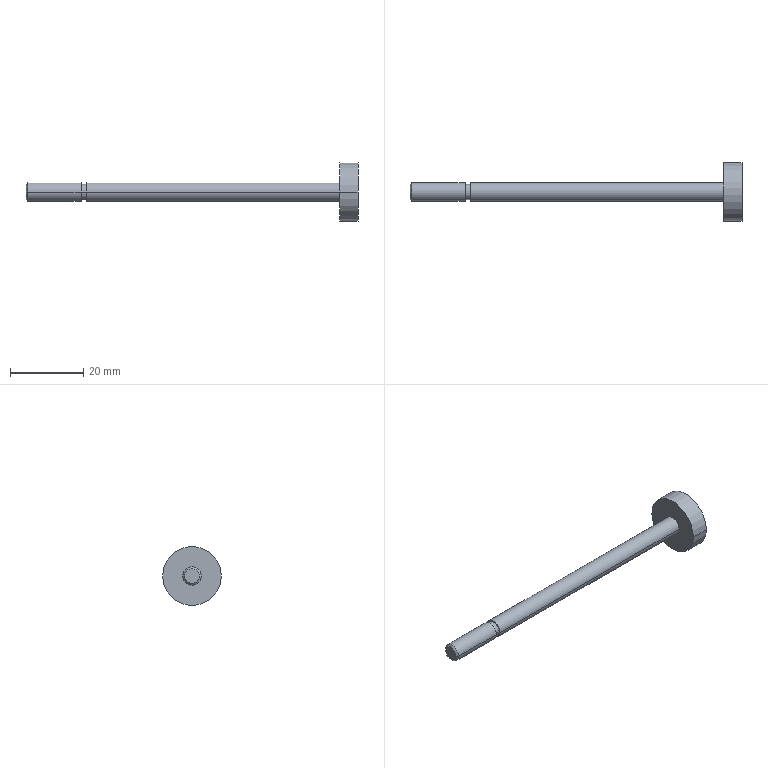Part | SolidWorks | features RefAxis 12, 3DProfileFeature 4, Revolution 1 | 1 solid | 15 faces | box 90.5 x 16 x 16 mm | volume 2673 mm3 | cylinder 8 | plane 5 | cone 2 | commonest cylinder face diameters 5 x4 4.13 x2 16 x2
STEP:
#1=CARTESIAN_POINT('',(90.5,-8.,0.));
#2=VERTEX_POINT('',#1);
#3=CARTESIAN_POINT('',(90.5,8.,0.));
#4=VERTEX_POINT('',#3);
#5=CARTESIAN_POINT('',(90.5,0.,0.));
#6=DIRECTION('',(-1.,0.,0.));
#7=DIRECTION('',(0.,-1.,0.));
#8=AXIS2_PLACEMENT_3D('',#5,#6,#7);
#9=CIRCLE('',#8,8.);
#10=EDGE_CURVE('',#2,#4,#9,.T.);
#11=ORIENTED_EDGE('',*,*,#10,.T.);
#12=CARTESIAN_POINT('',(85.5,8.,0.));
#13=VERTEX_POINT('',#12);
#14=CARTESIAN_POINT('',(90.5,8.,0.));
#15=DIRECTION('',(-1.,0.,0.));
#16=VECTOR('',#15,1000.);
#17=LINE('',#14,#16);
#18=EDGE_CURVE('',#4,#13,#17,.T.);
#19=ORIENTED_EDGE('',*,*,#18,.T.);
#20=CARTESIAN_POINT('',(85.5,-8.,0.));
#21=VERTEX_POINT('',#20);
#22=CARTESIAN_POINT('',(85.5,0.,0.));
#23=DIRECTION('',(-1.,0.,0.));
#24=DIRECTION('',(0.,-1.,0.));
#25=AXIS2_PLACEMENT_3D('',#22,#23,#24);
#26=CIRCLE('',#25,8.);
#27=EDGE_CURVE('',#21,#13,#26,.T.);
#28=ORIENTED_EDGE('',*,*,#27,.F.);
#29=CARTESIAN_POINT('',(90.5,-8.,0.));
#30=DIRECTION('',(-1.,0.,0.));
#31=VECTOR('',#30,1000.);
#32=LINE('',#29,#31);
#33=EDGE_CURVE('',#2,#21,#32,.T.);
#34=ORIENTED_EDGE('',*,*,#33,.F.);
#35=EDGE_LOOP('',(#11,#19,#28,#34));
#36=FACE_OUTER_BOUND('',#35,.T.);
#37=CARTESIAN_POINT('',(90.5,0.,0.));
#38=DIRECTION('',(-1.,0.,0.));
#39=DIRECTION('',(0.,-1.,0.));
#40=AXIS2_PLACEMENT_3D('',#37,#38,#39);
#41=CYLINDRICAL_SURFACE('',#40,8.);
#42=ADVANCED_FACE('',(#36),#41,.T.);
#43=CARTESIAN_POINT('',(85.5,-2.5,0.));
#44=VERTEX_POINT('',#43);
#45=CARTESIAN_POINT('',(85.5,2.5,0.));
#46=VERTEX_POINT('',#45);
#47=CARTESIAN_POINT('',(85.5,0.,0.));
#48=DIRECTION('',(-1.,0.,0.));
#49=DIRECTION('',(0.,-1.,0.));
#50=AXIS2_PLACEMENT_3D('',#47,#48,#49);
#51=CIRCLE('',#50,2.5);
#52=EDGE_CURVE('',#44,#46,#51,.T.);
#53=ORIENTED_EDGE('',*,*,#52,.T.);
#54=CARTESIAN_POINT('',(16.5,2.5,0.));
#55=VERTEX_POINT('',#54);
#56=CARTESIAN_POINT('',(90.5,2.5,0.));
#57=DIRECTION('',(-1.,0.,0.));
#58=VECTOR('',#57,1000.);
#59=LINE('',#56,#58);
#60=EDGE_CURVE('',#46,#55,#59,.T.);
#61=ORIENTED_EDGE('',*,*,#60,.T.);
#62=CARTESIAN_POINT('',(16.5,-2.5,0.));
#63=VERTEX_POINT('',#62);
#64=CARTESIAN_POINT('',(16.5,0.,0.));
#65=DIRECTION('',(-1.,0.,0.));
#66=DIRECTION('',(0.,-1.,0.));
#67=AXIS2_PLACEMENT_3D('',#64,#65,#66);
#68=CIRCLE('',#67,2.5);
#69=EDGE_CURVE('',#63,#55,#68,.T.);
#70=ORIENTED_EDGE('',*,*,#69,.F.);
#71=CARTESIAN_POINT('',(90.5,-2.5,0.));
#72=DIRECTION('',(-1.,0.,0.));
#73=VECTOR('',#72,1000.);
#74=LINE('',#71,#73);
#75=EDGE_CURVE('',#44,#63,#74,.T.);
#76=ORIENTED_EDGE('',*,*,#75,.F.);
#77=EDGE_LOOP('',(#53,#61,#70,#76));
#78=FACE_OUTER_BOUND('',#77,.T.);
#79=CARTESIAN_POINT('',(90.5,0.,0.));
#80=DIRECTION('',(-1.,0.,0.));
#81=DIRECTION('',(0.,-1.,0.));
#82=AXIS2_PLACEMENT_3D('',#79,#80,#81);
#83=CYLINDRICAL_SURFACE('',#82,2.5);
#84=ADVANCED_FACE('',(#78),#83,.T.);
#85=CARTESIAN_POINT('',(16.5,-2.065,0.));
#86=VERTEX_POINT('',#85);
#87=CARTESIAN_POINT('',(16.5,2.065,0.));
#88=VERTEX_POINT('',#87);
#89=CARTESIAN_POINT('',(16.5,0.,0.));
#90=DIRECTION('',(-1.,0.,0.));
#91=DIRECTION('',(0.,-1.,0.));
#92=AXIS2_PLACEMENT_3D('',#89,#90,#91);
#93=CIRCLE('',#92,2.065);
#94=EDGE_CURVE('',#86,#88,#93,.T.);
#95=ORIENTED_EDGE('',*,*,#94,.T.);
#96=CARTESIAN_POINT('',(15.,2.065,0.));
#97=VERTEX_POINT('',#96);
#98=CARTESIAN_POINT('',(90.5,2.065,0.));
#99=DIRECTION('',(-1.,0.,0.));
#100=VECTOR('',#99,1000.);
#101=LINE('',#98,#100);
#102=EDGE_CURVE('',#88,#97,#101,.T.);
#103=ORIENTED_EDGE('',*,*,#102,.T.);
#104=CARTESIAN_POINT('',(15.,-2.065,0.));
#105=VERTEX_POINT('',#104);
#106=CARTESIAN_POINT('',(15.,0.,0.));
#107=DIRECTION('',(-1.,0.,0.));
#108=DIRECTION('',(0.,-1.,0.));
#109=AXIS2_PLACEMENT_3D('',#106,#107,#108);
#110=CIRCLE('',#109,2.065);
#111=EDGE_CURVE('',#105,#97,#110,.T.);
#112=ORIENTED_EDGE('',*,*,#111,.F.);
#113=CARTESIAN_POINT('',(90.5,-2.065,0.));
#114=DIRECTION('',(-1.,0.,0.));
#115=VECTOR('',#114,1000.);
#116=LINE('',#113,#115);
#117=EDGE_CURVE('',#86,#105,#116,.T.);
#118=ORIENTED_EDGE('',*,*,#117,.F.);
#119=EDGE_LOOP('',(#95,#103,#112,#118));
#120=FACE_OUTER_BOUND('',#119,.T.);
#121=CARTESIAN_POINT('',(90.5,0.,0.));
#122=DIRECTION('',(-1.,0.,0.));
#123=DIRECTION('',(0.,-1.,0.));
#124=AXIS2_PLACEMENT_3D('',#121,#122,#123);
#125=CYLINDRICAL_SURFACE('',#124,2.065);
#126=ADVANCED_FACE('',(#120),#125,.T.);
#127=CARTESIAN_POINT('',(15.,-2.5,0.));
#128=VERTEX_POINT('',#127);
#129=CARTESIAN_POINT('',(15.,2.5,0.));
#130=VERTEX_POINT('',#129);
#131=CARTESIAN_POINT('',(15.,0.,0.));
#132=DIRECTION('',(-1.,0.,0.));
#133=DIRECTION('',(0.,-1.,0.));
#134=AXIS2_PLACEMENT_3D('',#131,#132,#133);
#135=CIRCLE('',#134,2.5);
#136=EDGE_CURVE('',#128,#130,#135,.T.);
#137=ORIENTED_EDGE('',*,*,#136,.T.);
#138=CARTESIAN_POINT('',(0.4905,2.5,0.));
#139=VERTEX_POINT('',#138);
#140=CARTESIAN_POINT('',(90.5,2.5,0.));
#141=DIRECTION('',(-1.,0.,0.));
#142=VECTOR('',#141,1000.);
#143=LINE('',#140,#142);
#144=EDGE_CURVE('',#130,#139,#143,.T.);
#145=ORIENTED_EDGE('',*,*,#144,.T.);
#146=CARTESIAN_POINT('',(0.4905,-2.5,0.));
#147=VERTEX_POINT('',#146);
#148=CARTESIAN_POINT('',(0.4905,0.,0.));
#149=DIRECTION('',(-1.,0.,0.));
#150=DIRECTION('',(0.,-1.,0.));
#151=AXIS2_PLACEMENT_3D('',#148,#149,#150);
#152=CIRCLE('',#151,2.5);
#153=EDGE_CURVE('',#147,#139,#152,.T.);
#154=ORIENTED_EDGE('',*,*,#153,.F.);
#155=CARTESIAN_POINT('',(90.5,-2.5,0.));
#156=DIRECTION('',(-1.,0.,0.));
#157=VECTOR('',#156,1000.);
#158=LINE('',#155,#157);
#159=EDGE_CURVE('',#128,#147,#158,.T.);
#160=ORIENTED_EDGE('',*,*,#159,.F.);
#161=EDGE_LOOP('',(#137,#145,#154,#160));
#162=FACE_OUTER_BOUND('',#161,.T.);
#163=CARTESIAN_POINT('',(90.5,0.,0.));
#164=DIRECTION('',(-1.,0.,0.));
#165=DIRECTION('',(0.,-1.,0.));
#166=AXIS2_PLACEMENT_3D('',#163,#164,#165);
#167=CYLINDRICAL_SURFACE('',#166,2.5);
#168=ADVANCED_FACE('',(#162),#167,.T.);
#169=CARTESIAN_POINT('',(0.,-2.01,0.));
#170=VERTEX_POINT('',#169);
#171=CARTESIAN_POINT('',(0.,2.01,0.));
#172=VERTEX_POINT('',#171);
#173=CARTESIAN_POINT('',(0.,0.,0.));
#174=DIRECTION('',(-1.,0.,0.));
#175=DIRECTION('',(0.,-1.,0.));
#176=AXIS2_PLACEMENT_3D('',#173,#174,#175);
#177=CIRCLE('',#176,2.01);
#178=EDGE_CURVE('',#170,#172,#177,.T.);
#179=ORIENTED_EDGE('',*,*,#178,.F.);
#180=CARTESIAN_POINT('',(0.4905,-2.5,0.));
#181=DIRECTION('',(0.7071,-0.7071,0.));
#182=VECTOR('',#181,1000.);
#183=LINE('',#180,#182);
#184=EDGE_CURVE('',#170,#147,#183,.T.);
#185=ORIENTED_EDGE('',*,*,#184,.T.);
#186=ORIENTED_EDGE('',*,*,#153,.T.);
#187=CARTESIAN_POINT('',(0.4905,2.5,0.));
#188=DIRECTION('',(0.7071,0.7071,0.));
#189=VECTOR('',#188,1000.);
#190=LINE('',#187,#189);
#191=EDGE_CURVE('',#172,#139,#190,.T.);
#192=ORIENTED_EDGE('',*,*,#191,.F.);
#193=EDGE_LOOP('',(#179,#185,#186,#192));
#194=FACE_OUTER_BOUND('',#193,.T.);
#195=CARTESIAN_POINT('',(0.4905,0.,0.));
#196=DIRECTION('',(1.,0.,0.));
#197=DIRECTION('',(0.,1.,0.));
#198=AXIS2_PLACEMENT_3D('',#195,#196,#197);
#199=CONICAL_SURFACE('',#198,2.5,0.7854);
#200=ADVANCED_FACE('',(#194),#199,.T.);
#201=CARTESIAN_POINT('',(0.,0.,0.));
#202=DIRECTION('',(-1.,0.,0.));
#203=DIRECTION('',(0.,-1.,0.));
#204=AXIS2_PLACEMENT_3D('',#201,#202,#203);
#205=CIRCLE('',#204,2.01);
#206=EDGE_CURVE('',#172,#170,#205,.T.);
#207=ORIENTED_EDGE('',*,*,#206,.T.);
#208=ORIENTED_EDGE('',*,*,#178,.T.);
#209=EDGE_LOOP('',(#207,#208));
#210=FACE_OUTER_BOUND('',#209,.T.);
#211=CARTESIAN_POINT('',(0.,0.,0.));
#212=DIRECTION('',(1.,0.,0.));
#213=DIRECTION('',(0.,1.,0.));
#214=AXIS2_PLACEMENT_3D('',#211,#212,#213);
#215=PLANE('',#214);
#216=ADVANCED_FACE('',(#210),#215,.F.);
#217=ORIENTED_EDGE('',*,*,#184,.F.);
#218=ORIENTED_EDGE('',*,*,#206,.F.);
#219=ORIENTED_EDGE('',*,*,#191,.T.);
#220=CARTESIAN_POINT('',(0.4905,0.,0.));
#221=DIRECTION('',(-1.,0.,0.));
#222=DIRECTION('',(0.,-1.,0.));
#223=AXIS2_PLACEMENT_3D('',#220,#221,#222);
#224=CIRCLE('',#223,2.5);
#225=EDGE_CURVE('',#139,#147,#224,.T.);
#226=ORIENTED_EDGE('',*,*,#225,.T.);
#227=EDGE_LOOP('',(#217,#218,#219,#226));
#228=FACE_OUTER_BOUND('',#227,.T.);
#229=CARTESIAN_POINT('',(0.4905,0.,0.));
#230=DIRECTION('',(1.,0.,0.));
#231=DIRECTION('',(0.,1.,0.));
#232=AXIS2_PLACEMENT_3D('',#229,#230,#231);
#233=CONICAL_SURFACE('',#232,2.5,0.7854);
#234=ADVANCED_FACE('',(#228),#233,.T.);
#235=ORIENTED_EDGE('',*,*,#144,.F.);
#236=CARTESIAN_POINT('',(15.,0.,0.));
#237=DIRECTION('',(-1.,0.,0.));
#238=DIRECTION('',(0.,-1.,0.));
#239=AXIS2_PLACEMENT_3D('',#236,#237,#238);
#240=CIRCLE('',#239,2.5);
#241=EDGE_CURVE('',#130,#128,#240,.T.);
#242=ORIENTED_EDGE('',*,*,#241,.T.);
#243=ORIENTED_EDGE('',*,*,#159,.T.);
#244=ORIENTED_EDGE('',*,*,#225,.F.);
#245=EDGE_LOOP('',(#235,#242,#243,#244));
#246=FACE_OUTER_BOUND('',#245,.T.);
#247=CARTESIAN_POINT('',(90.5,0.,0.));
#248=DIRECTION('',(-1.,0.,0.));
#249=DIRECTION('',(0.,-1.,0.));
#250=AXIS2_PLACEMENT_3D('',#247,#248,#249);
#251=CYLINDRICAL_SURFACE('',#250,2.5);
#252=ADVANCED_FACE('',(#246),#251,.T.);
#253=ORIENTED_EDGE('',*,*,#136,.F.);
#254=ORIENTED_EDGE('',*,*,#241,.F.);
#255=EDGE_LOOP('',(#253,#254));
#256=FACE_OUTER_BOUND('',#255,.T.);
#257=ORIENTED_EDGE('',*,*,#111,.T.);
#258=CARTESIAN_POINT('',(15.,0.,0.));
#259=DIRECTION('',(-1.,0.,0.));
#260=DIRECTION('',(0.,-1.,0.));
#261=AXIS2_PLACEMENT_3D('',#258,#259,#260);
#262=CIRCLE('',#261,2.065);
#263=EDGE_CURVE('',#97,#105,#262,.T.);
#264=ORIENTED_EDGE('',*,*,#263,.T.);
#265=EDGE_LOOP('',(#257,#264));
#266=FACE_BOUND('',#265,.T.);
#267=CARTESIAN_POINT('',(15.,2.5,0.));
#268=DIRECTION('',(-1.,0.,0.));
#269=DIRECTION('',(0.,-1.,0.));
#270=AXIS2_PLACEMENT_3D('',#267,#268,#269);
#271=PLANE('',#270);
#272=ADVANCED_FACE('',(#256,#266),#271,.F.);
#273=ORIENTED_EDGE('',*,*,#102,.F.);
#274=CARTESIAN_POINT('',(16.5,0.,0.));
#275=DIRECTION('',(-1.,0.,0.));
#276=DIRECTION('',(0.,-1.,0.));
#277=AXIS2_PLACEMENT_3D('',#274,#275,#276);
#278=CIRCLE('',#277,2.065);
#279=EDGE_CURVE('',#88,#86,#278,.T.);
#280=ORIENTED_EDGE('',*,*,#279,.T.);
#281=ORIENTED_EDGE('',*,*,#117,.T.);
#282=ORIENTED_EDGE('',*,*,#263,.F.);
#283=EDGE_LOOP('',(#273,#280,#281,#282));
#284=FACE_OUTER_BOUND('',#283,.T.);
#285=CARTESIAN_POINT('',(90.5,0.,0.));
#286=DIRECTION('',(-1.,0.,0.));
#287=DIRECTION('',(0.,-1.,0.));
#288=AXIS2_PLACEMENT_3D('',#285,#286,#287);
#289=CYLINDRICAL_SURFACE('',#288,2.065);
#290=ADVANCED_FACE('',(#284),#289,.T.);
#291=ORIENTED_EDGE('',*,*,#94,.F.);
#292=ORIENTED_EDGE('',*,*,#279,.F.);
#293=EDGE_LOOP('',(#291,#292));
#294=FACE_BOUND('',#293,.T.);
#295=ORIENTED_EDGE('',*,*,#69,.T.);
#296=CARTESIAN_POINT('',(16.5,0.,0.));
#297=DIRECTION('',(-1.,0.,0.));
#298=DIRECTION('',(0.,-1.,0.));
#299=AXIS2_PLACEMENT_3D('',#296,#297,#298);
#300=CIRCLE('',#299,2.5);
#301=EDGE_CURVE('',#55,#63,#300,.T.);
#302=ORIENTED_EDGE('',*,*,#301,.T.);
#303=EDGE_LOOP('',(#295,#302));
#304=FACE_OUTER_BOUND('',#303,.T.);
#305=CARTESIAN_POINT('',(16.5,2.065,0.));
#306=DIRECTION('',(1.,0.,0.));
#307=DIRECTION('',(0.,1.,0.));
#308=AXIS2_PLACEMENT_3D('',#305,#306,#307);
#309=PLANE('',#308);
#310=ADVANCED_FACE('',(#294,#304),#309,.F.);
#311=ORIENTED_EDGE('',*,*,#60,.F.);
#312=CARTESIAN_POINT('',(85.5,0.,0.));
#313=DIRECTION('',(-1.,0.,0.));
#314=DIRECTION('',(0.,-1.,0.));
#315=AXIS2_PLACEMENT_3D('',#312,#313,#314);
#316=CIRCLE('',#315,2.5);
#317=EDGE_CURVE('',#46,#44,#316,.T.);
#318=ORIENTED_EDGE('',*,*,#317,.T.);
#319=ORIENTED_EDGE('',*,*,#75,.T.);
#320=ORIENTED_EDGE('',*,*,#301,.F.);
#321=EDGE_LOOP('',(#311,#318,#319,#320));
#322=FACE_OUTER_BOUND('',#321,.T.);
#323=CARTESIAN_POINT('',(90.5,0.,0.));
#324=DIRECTION('',(-1.,0.,0.));
#325=DIRECTION('',(0.,-1.,0.));
#326=AXIS2_PLACEMENT_3D('',#323,#324,#325);
#327=CYLINDRICAL_SURFACE('',#326,2.5);
#328=ADVANCED_FACE('',(#322),#327,.T.);
#329=ORIENTED_EDGE('',*,*,#52,.F.);
#330=ORIENTED_EDGE('',*,*,#317,.F.);
#331=EDGE_LOOP('',(#329,#330));
#332=FACE_BOUND('',#331,.T.);
#333=ORIENTED_EDGE('',*,*,#27,.T.);
#334=CARTESIAN_POINT('',(85.5,0.,0.));
#335=DIRECTION('',(-1.,0.,0.));
#336=DIRECTION('',(0.,-1.,0.));
#337=AXIS2_PLACEMENT_3D('',#334,#335,#336);
#338=CIRCLE('',#337,8.);
#339=EDGE_CURVE('',#13,#21,#338,.T.);
#340=ORIENTED_EDGE('',*,*,#339,.T.);
#341=EDGE_LOOP('',(#333,#340));
#342=FACE_OUTER_BOUND('',#341,.T.);
#343=CARTESIAN_POINT('',(85.5,2.5,0.));
#344=DIRECTION('',(1.,0.,0.));
#345=DIRECTION('',(0.,1.,0.));
#346=AXIS2_PLACEMENT_3D('',#343,#344,#345);
#347=PLANE('',#346);
#348=ADVANCED_FACE('',(#332,#342),#347,.F.);
#349=ORIENTED_EDGE('',*,*,#18,.F.);
#350=CARTESIAN_POINT('',(90.5,0.,0.));
#351=DIRECTION('',(-1.,0.,0.));
#352=DIRECTION('',(0.,-1.,0.));
#353=AXIS2_PLACEMENT_3D('',#350,#351,#352);
#354=CIRCLE('',#353,8.);
#355=EDGE_CURVE('',#4,#2,#354,.T.);
#356=ORIENTED_EDGE('',*,*,#355,.T.);
#357=ORIENTED_EDGE('',*,*,#33,.T.);
#358=ORIENTED_EDGE('',*,*,#339,.F.);
#359=EDGE_LOOP('',(#349,#356,#357,#358));
#360=FACE_OUTER_BOUND('',#359,.T.);
#361=CARTESIAN_POINT('',(90.5,0.,0.));
#362=DIRECTION('',(-1.,0.,0.));
#363=DIRECTION('',(0.,-1.,0.));
#364=AXIS2_PLACEMENT_3D('',#361,#362,#363);
#365=CYLINDRICAL_SURFACE('',#364,8.);
#366=ADVANCED_FACE('',(#360),#365,.T.);
#367=ORIENTED_EDGE('',*,*,#10,.F.);
#368=ORIENTED_EDGE('',*,*,#355,.F.);
#369=EDGE_LOOP('',(#367,#368));
#370=FACE_OUTER_BOUND('',#369,.T.);
#371=CARTESIAN_POINT('',(90.5,8.,0.));
#372=DIRECTION('',(-1.,0.,0.));
#373=DIRECTION('',(0.,-1.,0.));
#374=AXIS2_PLACEMENT_3D('',#371,#372,#373);
#375=PLANE('',#374);
#376=ADVANCED_FACE('',(#370),#375,.F.);
#377=CLOSED_SHELL('',(#42,#84,#126,#168,#200,#216,#234,#252,#272,#290,#310,#328,#348,#366,#376));
#378=MANIFOLD_SOLID_BREP('',#377);
#379=CARTESIAN_POINT('',(0.,0.,0.));
#380=DIRECTION('',(0.,0.,1.));
#381=DIRECTION('',(1.,0.,0.));
#382=AXIS2_PLACEMENT_3D('',#379,#380,#381);
#383=(LENGTH_UNIT()NAMED_UNIT(*)SI_UNIT(.MILLI.,.METRE.));
#384=UNCERTAINTY_MEASURE_WITH_UNIT(LENGTH_MEASURE(0.00001),#383,'','');
#385=(NAMED_UNIT(*)PLANE_ANGLE_UNIT()SI_UNIT($,.RADIAN.));
#386=(NAMED_UNIT(*)SI_UNIT($,.STERADIAN.)SOLID_ANGLE_UNIT());
#387=(GEOMETRIC_REPRESENTATION_CONTEXT(3)GLOBAL_UNCERTAINTY_ASSIGNED_CONTEXT((#384))GLOBAL_UNIT_ASSIGNED_CONTEXT((#383,#385,#386))REPRESENTATION_CONTEXT('',''));
#388=ADVANCED_BREP_SHAPE_REPRESENTATION('',(#378,#382),#387);